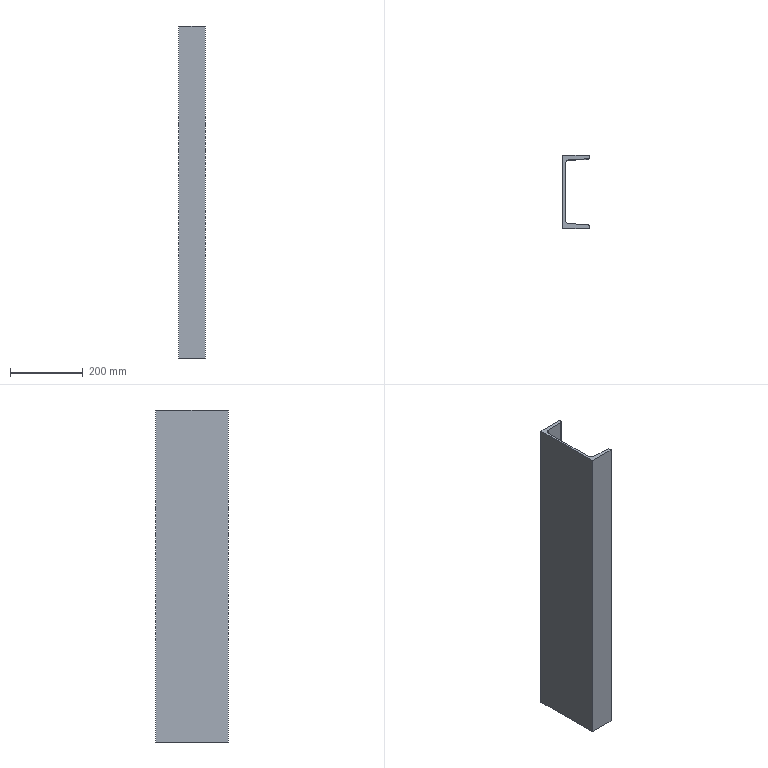Part | SolidWorks | features Extrusion 1 | 1 solid | 14 faces | box 73 x 200 x 914.4 mm | volume 2618794 mm3 | plane 10 | cylinder 4 | commonest cylinder face diameters 11 x2 22 x2
STEP:
#1=CARTESIAN_POINT('',(73.,200.,-457.2));
#2=VERTEX_POINT('',#1);
#3=CARTESIAN_POINT('',(0.,200.,-457.2));
#4=VERTEX_POINT('',#3);
#5=CARTESIAN_POINT('',(0.,200.,-457.2));
#6=DIRECTION('',(-1.,0.,0.));
#7=VECTOR('',#6,1000.);
#8=LINE('',#5,#7);
#9=EDGE_CURVE('',#2,#4,#8,.T.);
#10=ORIENTED_EDGE('',*,*,#9,.T.);
#11=CARTESIAN_POINT('',(0.,200.,457.2));
#12=VERTEX_POINT('',#11);
#13=CARTESIAN_POINT('',(0.,200.,457.2));
#14=DIRECTION('',(0.,0.,-1.));
#15=VECTOR('',#14,1000.);
#16=LINE('',#13,#15);
#17=EDGE_CURVE('',#12,#4,#16,.T.);
#18=ORIENTED_EDGE('',*,*,#17,.F.);
#19=CARTESIAN_POINT('',(73.,200.,457.2));
#20=VERTEX_POINT('',#19);
#21=CARTESIAN_POINT('',(0.,200.,457.2));
#22=DIRECTION('',(-1.,0.,0.));
#23=VECTOR('',#22,1000.);
#24=LINE('',#21,#23);
#25=EDGE_CURVE('',#20,#12,#24,.T.);
#26=ORIENTED_EDGE('',*,*,#25,.F.);
#27=CARTESIAN_POINT('',(73.,200.,457.2));
#28=DIRECTION('',(0.,0.,-1.));
#29=VECTOR('',#28,1000.);
#30=LINE('',#27,#29);
#31=EDGE_CURVE('',#20,#2,#30,.T.);
#32=ORIENTED_EDGE('',*,*,#31,.T.);
#33=EDGE_LOOP('',(#10,#18,#26,#32));
#34=FACE_OUTER_BOUND('',#33,.T.);
#35=CARTESIAN_POINT('',(0.,200.,457.2));
#36=DIRECTION('',(0.,-1.,0.));
#37=DIRECTION('',(0.,0.,-1.));
#38=AXIS2_PLACEMENT_3D('',#35,#36,#37);
#39=PLANE('',#38);
#40=ADVANCED_FACE('',(#34),#39,.F.);
#41=CARTESIAN_POINT('',(0.,0.,-457.2));
#42=VERTEX_POINT('',#41);
#43=CARTESIAN_POINT('',(0.,0.,-457.2));
#44=DIRECTION('',(0.,-1.,0.));
#45=VECTOR('',#44,1000.);
#46=LINE('',#43,#45);
#47=EDGE_CURVE('',#4,#42,#46,.T.);
#48=ORIENTED_EDGE('',*,*,#47,.T.);
#49=CARTESIAN_POINT('',(0.,0.,457.2));
#50=VERTEX_POINT('',#49);
#51=CARTESIAN_POINT('',(0.,0.,457.2));
#52=DIRECTION('',(0.,0.,-1.));
#53=VECTOR('',#52,1000.);
#54=LINE('',#51,#53);
#55=EDGE_CURVE('',#50,#42,#54,.T.);
#56=ORIENTED_EDGE('',*,*,#55,.F.);
#57=CARTESIAN_POINT('',(0.,0.,457.2));
#58=DIRECTION('',(0.,-1.,0.));
#59=VECTOR('',#58,1000.);
#60=LINE('',#57,#59);
#61=EDGE_CURVE('',#12,#50,#60,.T.);
#62=ORIENTED_EDGE('',*,*,#61,.F.);
#63=ORIENTED_EDGE('',*,*,#17,.T.);
#64=EDGE_LOOP('',(#48,#56,#62,#63));
#65=FACE_OUTER_BOUND('',#64,.T.);
#66=CARTESIAN_POINT('',(0.,0.,457.2));
#67=DIRECTION('',(1.,0.,0.));
#68=DIRECTION('',(0.,0.,-1.));
#69=AXIS2_PLACEMENT_3D('',#66,#67,#68);
#70=PLANE('',#69);
#71=ADVANCED_FACE('',(#65),#70,.F.);
#72=CARTESIAN_POINT('',(73.,0.,-457.2));
#73=VERTEX_POINT('',#72);
#74=CARTESIAN_POINT('',(0.,0.,-457.2));
#75=DIRECTION('',(1.,0.,0.));
#76=VECTOR('',#75,1000.);
#77=LINE('',#74,#76);
#78=EDGE_CURVE('',#42,#73,#77,.T.);
#79=ORIENTED_EDGE('',*,*,#78,.T.);
#80=CARTESIAN_POINT('',(73.,0.,457.2));
#81=VERTEX_POINT('',#80);
#82=CARTESIAN_POINT('',(73.,0.,457.2));
#83=DIRECTION('',(0.,0.,-1.));
#84=VECTOR('',#83,1000.);
#85=LINE('',#82,#84);
#86=EDGE_CURVE('',#81,#73,#85,.T.);
#87=ORIENTED_EDGE('',*,*,#86,.F.);
#88=CARTESIAN_POINT('',(0.,0.,457.2));
#89=DIRECTION('',(1.,0.,0.));
#90=VECTOR('',#89,1000.);
#91=LINE('',#88,#90);
#92=EDGE_CURVE('',#50,#81,#91,.T.);
#93=ORIENTED_EDGE('',*,*,#92,.F.);
#94=ORIENTED_EDGE('',*,*,#55,.T.);
#95=EDGE_LOOP('',(#79,#87,#93,#94));
#96=FACE_OUTER_BOUND('',#95,.T.);
#97=CARTESIAN_POINT('',(0.,0.,457.2));
#98=DIRECTION('',(0.,1.,0.));
#99=DIRECTION('',(0.,0.,1.));
#100=AXIS2_PLACEMENT_3D('',#97,#98,#99);
#101=PLANE('',#100);
#102=ADVANCED_FACE('',(#96),#101,.F.);
#103=CARTESIAN_POINT('',(73.,3.967,-457.2));
#104=VERTEX_POINT('',#103);
#105=CARTESIAN_POINT('',(73.,3.967,-457.2));
#106=DIRECTION('',(0.,1.,0.));
#107=VECTOR('',#106,1000.);
#108=LINE('',#105,#107);
#109=EDGE_CURVE('',#73,#104,#108,.T.);
#110=ORIENTED_EDGE('',*,*,#109,.T.);
#111=CARTESIAN_POINT('',(73.,3.967,457.2));
#112=VERTEX_POINT('',#111);
#113=CARTESIAN_POINT('',(73.,3.967,457.2));
#114=DIRECTION('',(0.,0.,-1.));
#115=VECTOR('',#114,1000.);
#116=LINE('',#113,#115);
#117=EDGE_CURVE('',#112,#104,#116,.T.);
#118=ORIENTED_EDGE('',*,*,#117,.F.);
#119=CARTESIAN_POINT('',(73.,3.967,457.2));
#120=DIRECTION('',(0.,1.,0.));
#121=VECTOR('',#120,1000.);
#122=LINE('',#119,#121);
#123=EDGE_CURVE('',#81,#112,#122,.T.);
#124=ORIENTED_EDGE('',*,*,#123,.F.);
#125=ORIENTED_EDGE('',*,*,#86,.T.);
#126=EDGE_LOOP('',(#110,#118,#124,#125));
#127=FACE_OUTER_BOUND('',#126,.T.);
#128=CARTESIAN_POINT('',(73.,3.967,457.2));
#129=DIRECTION('',(-1.,0.,0.));
#130=DIRECTION('',(0.,-1.,0.));
#131=AXIS2_PLACEMENT_3D('',#128,#129,#130);
#132=PLANE('',#131);
#133=ADVANCED_FACE('',(#127),#132,.F.);
#134=CARTESIAN_POINT('',(67.771,9.46,-457.2));
#135=VERTEX_POINT('',#134);
#136=CARTESIAN_POINT('',(67.5,3.967,-457.2));
#137=DIRECTION('',(0.,0.,1.));
#138=DIRECTION('',(1.,0.,0.));
#139=AXIS2_PLACEMENT_3D('',#136,#137,#138);
#140=CIRCLE('',#139,5.5);
#141=EDGE_CURVE('',#104,#135,#140,.T.);
#142=ORIENTED_EDGE('',*,*,#141,.T.);
#143=CARTESIAN_POINT('',(67.771,9.46,457.2));
#144=VERTEX_POINT('',#143);
#145=CARTESIAN_POINT('',(67.771,9.46,457.2));
#146=DIRECTION('',(0.,0.,-1.));
#147=VECTOR('',#146,1000.);
#148=LINE('',#145,#147);
#149=EDGE_CURVE('',#144,#135,#148,.T.);
#150=ORIENTED_EDGE('',*,*,#149,.F.);
#151=CARTESIAN_POINT('',(67.5,3.967,457.2));
#152=DIRECTION('',(0.,0.,1.));
#153=DIRECTION('',(1.,0.,0.));
#154=AXIS2_PLACEMENT_3D('',#151,#152,#153);
#155=CIRCLE('',#154,5.5);
#156=EDGE_CURVE('',#112,#144,#155,.T.);
#157=ORIENTED_EDGE('',*,*,#156,.F.);
#158=ORIENTED_EDGE('',*,*,#117,.T.);
#159=EDGE_LOOP('',(#142,#150,#157,#158));
#160=FACE_OUTER_BOUND('',#159,.T.);
#161=CARTESIAN_POINT('',(67.5,3.967,457.2));
#162=DIRECTION('',(0.,0.,-1.));
#163=DIRECTION('',(-1.,0.,0.));
#164=AXIS2_PLACEMENT_3D('',#161,#162,#163);
#165=CYLINDRICAL_SURFACE('',#164,5.5);
#166=ADVANCED_FACE('',(#160),#165,.T.);
#167=CARTESIAN_POINT('',(17.459,11.938,-457.2));
#168=VERTEX_POINT('',#167);
#169=CARTESIAN_POINT('',(17.459,11.938,-457.2));
#170=DIRECTION('',(-0.9988,0.04918,0.));
#171=VECTOR('',#170,1000.);
#172=LINE('',#169,#171);
#173=EDGE_CURVE('',#135,#168,#172,.T.);
#174=ORIENTED_EDGE('',*,*,#173,.T.);
#175=CARTESIAN_POINT('',(17.459,11.938,457.2));
#176=VERTEX_POINT('',#175);
#177=CARTESIAN_POINT('',(17.459,11.938,457.2));
#178=DIRECTION('',(0.,0.,-1.));
#179=VECTOR('',#178,1000.);
#180=LINE('',#177,#179);
#181=EDGE_CURVE('',#176,#168,#180,.T.);
#182=ORIENTED_EDGE('',*,*,#181,.F.);
#183=CARTESIAN_POINT('',(17.459,11.938,457.2));
#184=DIRECTION('',(-0.9988,0.04918,0.));
#185=VECTOR('',#184,1000.);
#186=LINE('',#183,#185);
#187=EDGE_CURVE('',#144,#176,#186,.T.);
#188=ORIENTED_EDGE('',*,*,#187,.F.);
#189=ORIENTED_EDGE('',*,*,#149,.T.);
#190=EDGE_LOOP('',(#174,#182,#188,#189));
#191=FACE_OUTER_BOUND('',#190,.T.);
#192=CARTESIAN_POINT('',(17.459,11.938,457.2));
#193=DIRECTION('',(-0.04918,-0.9988,0.));
#194=DIRECTION('',(0.9988,-0.04918,0.));
#195=AXIS2_PLACEMENT_3D('',#192,#193,#194);
#196=PLANE('',#195);
#197=ADVANCED_FACE('',(#191),#196,.F.);
#198=CARTESIAN_POINT('',(7.,22.924,-457.2));
#199=VERTEX_POINT('',#198);
#200=CARTESIAN_POINT('',(18.,22.924,-457.2));
#201=DIRECTION('',(0.,0.,-1.));
#202=DIRECTION('',(-1.,0.,0.));
#203=AXIS2_PLACEMENT_3D('',#200,#201,#202);
#204=CIRCLE('',#203,11.);
#205=EDGE_CURVE('',#168,#199,#204,.T.);
#206=ORIENTED_EDGE('',*,*,#205,.T.);
#207=CARTESIAN_POINT('',(7.,22.924,457.2));
#208=VERTEX_POINT('',#207);
#209=CARTESIAN_POINT('',(7.,22.924,457.2));
#210=DIRECTION('',(0.,0.,-1.));
#211=VECTOR('',#210,1000.);
#212=LINE('',#209,#211);
#213=EDGE_CURVE('',#208,#199,#212,.T.);
#214=ORIENTED_EDGE('',*,*,#213,.F.);
#215=CARTESIAN_POINT('',(18.,22.924,457.2));
#216=DIRECTION('',(0.,0.,-1.));
#217=DIRECTION('',(-1.,0.,0.));
#218=AXIS2_PLACEMENT_3D('',#215,#216,#217);
#219=CIRCLE('',#218,11.);
#220=EDGE_CURVE('',#176,#208,#219,.T.);
#221=ORIENTED_EDGE('',*,*,#220,.F.);
#222=ORIENTED_EDGE('',*,*,#181,.T.);
#223=EDGE_LOOP('',(#206,#214,#221,#222));
#224=FACE_OUTER_BOUND('',#223,.T.);
#225=CARTESIAN_POINT('',(18.,22.924,457.2));
#226=DIRECTION('',(0.,0.,-1.));
#227=DIRECTION('',(-1.,0.,0.));
#228=AXIS2_PLACEMENT_3D('',#225,#226,#227);
#229=CYLINDRICAL_SURFACE('',#228,11.);
#230=ADVANCED_FACE('',(#224),#229,.F.);
#231=CARTESIAN_POINT('',(7.,177.076,-457.2));
#232=VERTEX_POINT('',#231);
#233=CARTESIAN_POINT('',(7.,177.076,-457.2));
#234=DIRECTION('',(0.,1.,0.));
#235=VECTOR('',#234,1000.);
#236=LINE('',#233,#235);
#237=EDGE_CURVE('',#199,#232,#236,.T.);
#238=ORIENTED_EDGE('',*,*,#237,.T.);
#239=CARTESIAN_POINT('',(7.,177.076,457.2));
#240=VERTEX_POINT('',#239);
#241=CARTESIAN_POINT('',(7.,177.076,457.2));
#242=DIRECTION('',(0.,0.,-1.));
#243=VECTOR('',#242,1000.);
#244=LINE('',#241,#243);
#245=EDGE_CURVE('',#240,#232,#244,.T.);
#246=ORIENTED_EDGE('',*,*,#245,.F.);
#247=CARTESIAN_POINT('',(7.,177.076,457.2));
#248=DIRECTION('',(0.,1.,0.));
#249=VECTOR('',#248,1000.);
#250=LINE('',#247,#249);
#251=EDGE_CURVE('',#208,#240,#250,.T.);
#252=ORIENTED_EDGE('',*,*,#251,.F.);
#253=ORIENTED_EDGE('',*,*,#213,.T.);
#254=EDGE_LOOP('',(#238,#246,#252,#253));
#255=FACE_OUTER_BOUND('',#254,.T.);
#256=CARTESIAN_POINT('',(7.,177.076,457.2));
#257=DIRECTION('',(-1.,0.,0.));
#258=DIRECTION('',(0.,0.,1.));
#259=AXIS2_PLACEMENT_3D('',#256,#257,#258);
#260=PLANE('',#259);
#261=ADVANCED_FACE('',(#255),#260,.F.);
#262=CARTESIAN_POINT('',(17.459,188.062,-457.2));
#263=VERTEX_POINT('',#262);
#264=CARTESIAN_POINT('',(18.,177.076,-457.2));
#265=DIRECTION('',(0.,0.,-1.));
#266=DIRECTION('',(-1.,0.,0.));
#267=AXIS2_PLACEMENT_3D('',#264,#265,#266);
#268=CIRCLE('',#267,11.);
#269=EDGE_CURVE('',#232,#263,#268,.T.);
#270=ORIENTED_EDGE('',*,*,#269,.T.);
#271=CARTESIAN_POINT('',(17.459,188.062,457.2));
#272=VERTEX_POINT('',#271);
#273=CARTESIAN_POINT('',(17.459,188.062,457.2));
#274=DIRECTION('',(0.,0.,-1.));
#275=VECTOR('',#274,1000.);
#276=LINE('',#273,#275);
#277=EDGE_CURVE('',#272,#263,#276,.T.);
#278=ORIENTED_EDGE('',*,*,#277,.F.);
#279=CARTESIAN_POINT('',(18.,177.076,457.2));
#280=DIRECTION('',(0.,0.,-1.));
#281=DIRECTION('',(-1.,0.,0.));
#282=AXIS2_PLACEMENT_3D('',#279,#280,#281);
#283=CIRCLE('',#282,11.);
#284=EDGE_CURVE('',#240,#272,#283,.T.);
#285=ORIENTED_EDGE('',*,*,#284,.F.);
#286=ORIENTED_EDGE('',*,*,#245,.T.);
#287=EDGE_LOOP('',(#270,#278,#285,#286));
#288=FACE_OUTER_BOUND('',#287,.T.);
#289=CARTESIAN_POINT('',(18.,177.076,457.2));
#290=DIRECTION('',(0.,0.,-1.));
#291=DIRECTION('',(-1.,0.,0.));
#292=AXIS2_PLACEMENT_3D('',#289,#290,#291);
#293=CYLINDRICAL_SURFACE('',#292,11.);
#294=ADVANCED_FACE('',(#288),#293,.F.);
#295=CARTESIAN_POINT('',(67.771,190.54,-457.2));
#296=VERTEX_POINT('',#295);
#297=CARTESIAN_POINT('',(17.459,188.062,-457.2));
#298=DIRECTION('',(0.9988,0.04918,0.));
#299=VECTOR('',#298,1000.);
#300=LINE('',#297,#299);
#301=EDGE_CURVE('',#263,#296,#300,.T.);
#302=ORIENTED_EDGE('',*,*,#301,.T.);
#303=CARTESIAN_POINT('',(67.771,190.54,457.2));
#304=VERTEX_POINT('',#303);
#305=CARTESIAN_POINT('',(67.771,190.54,457.2));
#306=DIRECTION('',(0.,0.,-1.));
#307=VECTOR('',#306,1000.);
#308=LINE('',#305,#307);
#309=EDGE_CURVE('',#304,#296,#308,.T.);
#310=ORIENTED_EDGE('',*,*,#309,.F.);
#311=CARTESIAN_POINT('',(17.459,188.062,457.2));
#312=DIRECTION('',(0.9988,0.04918,0.));
#313=VECTOR('',#312,1000.);
#314=LINE('',#311,#313);
#315=EDGE_CURVE('',#272,#304,#314,.T.);
#316=ORIENTED_EDGE('',*,*,#315,.F.);
#317=ORIENTED_EDGE('',*,*,#277,.T.);
#318=EDGE_LOOP('',(#302,#310,#316,#317));
#319=FACE_OUTER_BOUND('',#318,.T.);
#320=CARTESIAN_POINT('',(17.459,188.062,457.2));
#321=DIRECTION('',(-0.04918,0.9988,0.));
#322=DIRECTION('',(-0.9988,-0.04918,0.));
#323=AXIS2_PLACEMENT_3D('',#320,#321,#322);
#324=PLANE('',#323);
#325=ADVANCED_FACE('',(#319),#324,.F.);
#326=CARTESIAN_POINT('',(73.,196.033,-457.2));
#327=VERTEX_POINT('',#326);
#328=CARTESIAN_POINT('',(67.5,196.033,-457.2));
#329=DIRECTION('',(0.,0.,1.));
#330=DIRECTION('',(1.,0.,0.));
#331=AXIS2_PLACEMENT_3D('',#328,#329,#330);
#332=CIRCLE('',#331,5.5);
#333=EDGE_CURVE('',#296,#327,#332,.T.);
#334=ORIENTED_EDGE('',*,*,#333,.T.);
#335=CARTESIAN_POINT('',(73.,196.033,457.2));
#336=VERTEX_POINT('',#335);
#337=CARTESIAN_POINT('',(73.,196.033,457.2));
#338=DIRECTION('',(0.,0.,-1.));
#339=VECTOR('',#338,1000.);
#340=LINE('',#337,#339);
#341=EDGE_CURVE('',#336,#327,#340,.T.);
#342=ORIENTED_EDGE('',*,*,#341,.F.);
#343=CARTESIAN_POINT('',(67.5,196.033,457.2));
#344=DIRECTION('',(0.,0.,1.));
#345=DIRECTION('',(1.,0.,0.));
#346=AXIS2_PLACEMENT_3D('',#343,#344,#345);
#347=CIRCLE('',#346,5.5);
#348=EDGE_CURVE('',#304,#336,#347,.T.);
#349=ORIENTED_EDGE('',*,*,#348,.F.);
#350=ORIENTED_EDGE('',*,*,#309,.T.);
#351=EDGE_LOOP('',(#334,#342,#349,#350));
#352=FACE_OUTER_BOUND('',#351,.T.);
#353=CARTESIAN_POINT('',(67.5,196.033,457.2));
#354=DIRECTION('',(0.,0.,-1.));
#355=DIRECTION('',(-1.,0.,0.));
#356=AXIS2_PLACEMENT_3D('',#353,#354,#355);
#357=CYLINDRICAL_SURFACE('',#356,5.5);
#358=ADVANCED_FACE('',(#352),#357,.T.);
#359=CARTESIAN_POINT('',(73.,196.033,-457.2));
#360=DIRECTION('',(0.,1.,0.));
#361=VECTOR('',#360,1000.);
#362=LINE('',#359,#361);
#363=EDGE_CURVE('',#327,#2,#362,.T.);
#364=ORIENTED_EDGE('',*,*,#363,.T.);
#365=ORIENTED_EDGE('',*,*,#31,.F.);
#366=CARTESIAN_POINT('',(73.,196.033,457.2));
#367=DIRECTION('',(0.,1.,0.));
#368=VECTOR('',#367,1000.);
#369=LINE('',#366,#368);
#370=EDGE_CURVE('',#336,#20,#369,.T.);
#371=ORIENTED_EDGE('',*,*,#370,.F.);
#372=ORIENTED_EDGE('',*,*,#341,.T.);
#373=EDGE_LOOP('',(#364,#365,#371,#372));
#374=FACE_OUTER_BOUND('',#373,.T.);
#375=CARTESIAN_POINT('',(73.,196.033,457.2));
#376=DIRECTION('',(-1.,0.,0.));
#377=DIRECTION('',(0.,-1.,0.));
#378=AXIS2_PLACEMENT_3D('',#375,#376,#377);
#379=PLANE('',#378);
#380=ADVANCED_FACE('',(#374),#379,.F.);
#381=ORIENTED_EDGE('',*,*,#25,.T.);
#382=ORIENTED_EDGE('',*,*,#61,.T.);
#383=ORIENTED_EDGE('',*,*,#92,.T.);
#384=ORIENTED_EDGE('',*,*,#123,.T.);
#385=ORIENTED_EDGE('',*,*,#156,.T.);
#386=ORIENTED_EDGE('',*,*,#187,.T.);
#387=ORIENTED_EDGE('',*,*,#220,.T.);
#388=ORIENTED_EDGE('',*,*,#251,.T.);
#389=ORIENTED_EDGE('',*,*,#284,.T.);
#390=ORIENTED_EDGE('',*,*,#315,.T.);
#391=ORIENTED_EDGE('',*,*,#348,.T.);
#392=ORIENTED_EDGE('',*,*,#370,.T.);
#393=EDGE_LOOP('',(#381,#382,#383,#384,#385,#386,#387,#388,#389,#390,#391,#392));
#394=FACE_OUTER_BOUND('',#393,.T.);
#395=CARTESIAN_POINT('',(67.5,196.033,457.2));
#396=DIRECTION('',(0.,0.,1.));
#397=DIRECTION('',(1.,0.,0.));
#398=AXIS2_PLACEMENT_3D('',#395,#396,#397);
#399=PLANE('',#398);
#400=ADVANCED_FACE('',(#394),#399,.T.);
#401=ORIENTED_EDGE('',*,*,#9,.F.);
#402=ORIENTED_EDGE('',*,*,#363,.F.);
#403=ORIENTED_EDGE('',*,*,#333,.F.);
#404=ORIENTED_EDGE('',*,*,#301,.F.);
#405=ORIENTED_EDGE('',*,*,#269,.F.);
#406=ORIENTED_EDGE('',*,*,#237,.F.);
#407=ORIENTED_EDGE('',*,*,#205,.F.);
#408=ORIENTED_EDGE('',*,*,#173,.F.);
#409=ORIENTED_EDGE('',*,*,#141,.F.);
#410=ORIENTED_EDGE('',*,*,#109,.F.);
#411=ORIENTED_EDGE('',*,*,#78,.F.);
#412=ORIENTED_EDGE('',*,*,#47,.F.);
#413=EDGE_LOOP('',(#401,#402,#403,#404,#405,#406,#407,#408,#409,#410,#411,#412));
#414=FACE_OUTER_BOUND('',#413,.T.);
#415=CARTESIAN_POINT('',(67.5,196.033,-457.2));
#416=DIRECTION('',(0.,0.,1.));
#417=DIRECTION('',(1.,0.,0.));
#418=AXIS2_PLACEMENT_3D('',#415,#416,#417);
#419=PLANE('',#418);
#420=ADVANCED_FACE('',(#414),#419,.F.);
#421=CLOSED_SHELL('',(#40,#71,#102,#133,#166,#197,#230,#261,#294,#325,#358,#380,#400,#420));
#422=MANIFOLD_SOLID_BREP('',#421);
#423=CARTESIAN_POINT('',(0.,0.,0.));
#424=DIRECTION('',(0.,0.,1.));
#425=DIRECTION('',(1.,0.,0.));
#426=AXIS2_PLACEMENT_3D('',#423,#424,#425);
#427=(LENGTH_UNIT()NAMED_UNIT(*)SI_UNIT(.MILLI.,.METRE.));
#428=UNCERTAINTY_MEASURE_WITH_UNIT(LENGTH_MEASURE(0.00001),#427,'','');
#429=(NAMED_UNIT(*)PLANE_ANGLE_UNIT()SI_UNIT($,.RADIAN.));
#430=(NAMED_UNIT(*)SI_UNIT($,.STERADIAN.)SOLID_ANGLE_UNIT());
#431=(GEOMETRIC_REPRESENTATION_CONTEXT(3)GLOBAL_UNCERTAINTY_ASSIGNED_CONTEXT((#428))GLOBAL_UNIT_ASSIGNED_CONTEXT((#427,#429,#430))REPRESENTATION_CONTEXT('',''));
#432=ADVANCED_BREP_SHAPE_REPRESENTATION('',(#422,#426),#431);